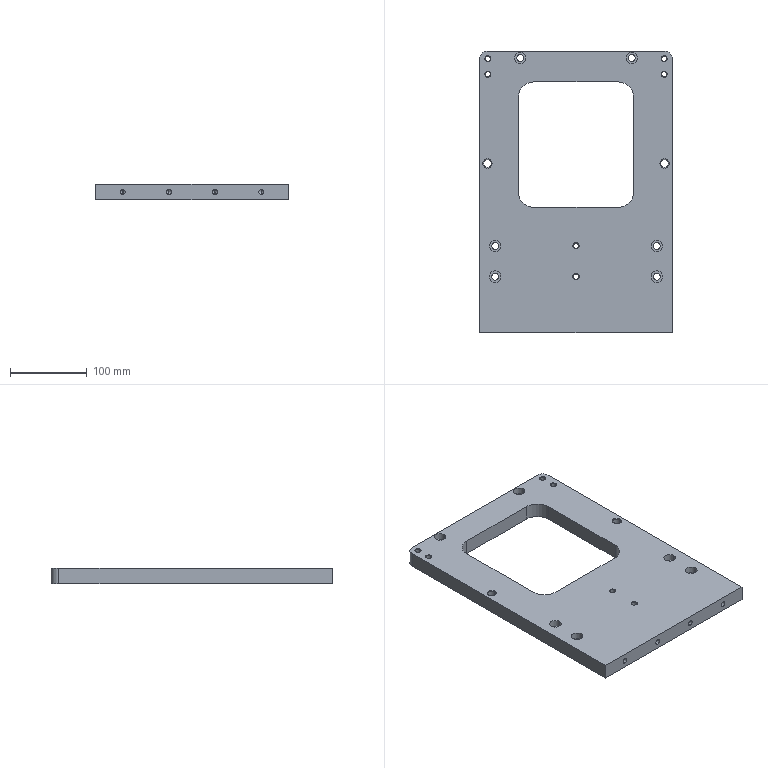Part | 1 solid | 94 faces | box 250 x 366 x 20 mm | volume 1322605 mm3 | cylinder 54 | cone 24 | plane 16 | commonest cylinder face diameters 6.8 x20 9 x12 15 x12 10.2 x4 40 x4 20 x2